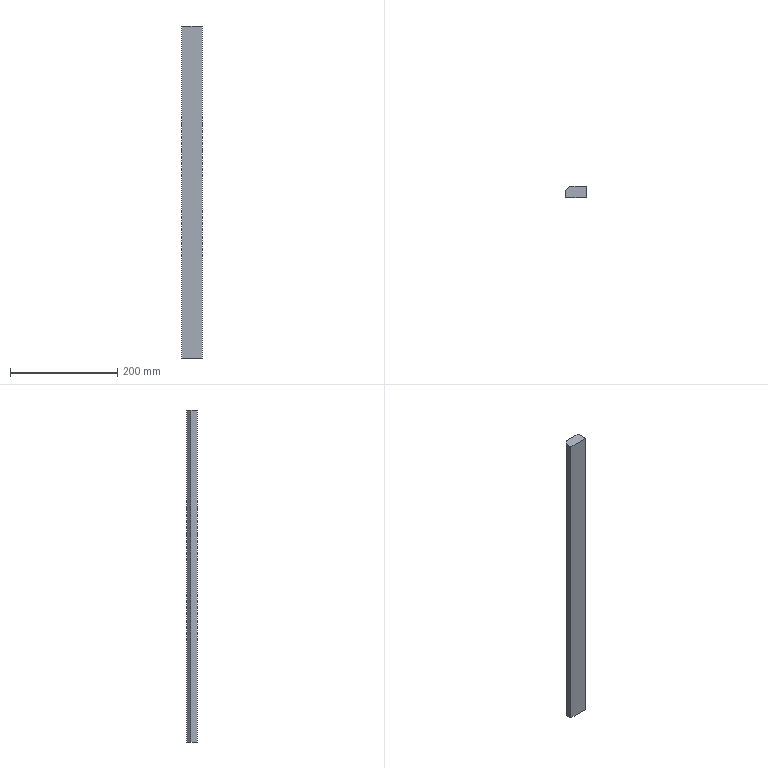Part | SolidWorks | features Chamfer 1, Extrusion 1 | 1 solid | 7 faces | box 39 x 20 x 620 mm | volume 463760 mm3 | plane 7
STEP:
#1=CARTESIAN_POINT('',(0.,12.,620.));
#2=VERTEX_POINT('',#1);
#3=CARTESIAN_POINT('',(0.,0.,620.));
#4=VERTEX_POINT('',#3);
#5=CARTESIAN_POINT('',(0.,0.,620.));
#6=DIRECTION('',(0.,-1.,0.));
#7=VECTOR('',#6,1000.);
#8=LINE('',#5,#7);
#9=EDGE_CURVE('',#2,#4,#8,.T.);
#10=ORIENTED_EDGE('',*,*,#9,.F.);
#11=CARTESIAN_POINT('',(0.,12.,0.));
#12=VERTEX_POINT('',#11);
#13=CARTESIAN_POINT('',(0.,12.,620.));
#14=DIRECTION('',(0.,0.,-1.));
#15=VECTOR('',#14,1000.);
#16=LINE('',#13,#15);
#17=EDGE_CURVE('',#2,#12,#16,.T.);
#18=ORIENTED_EDGE('',*,*,#17,.T.);
#19=CARTESIAN_POINT('',(0.,0.,0.));
#20=VERTEX_POINT('',#19);
#21=CARTESIAN_POINT('',(0.,0.,0.));
#22=DIRECTION('',(0.,-1.,0.));
#23=VECTOR('',#22,1000.);
#24=LINE('',#21,#23);
#25=EDGE_CURVE('',#12,#20,#24,.T.);
#26=ORIENTED_EDGE('',*,*,#25,.T.);
#27=CARTESIAN_POINT('',(0.,0.,620.));
#28=DIRECTION('',(0.,0.,-1.));
#29=VECTOR('',#28,1000.);
#30=LINE('',#27,#29);
#31=EDGE_CURVE('',#4,#20,#30,.T.);
#32=ORIENTED_EDGE('',*,*,#31,.F.);
#33=EDGE_LOOP('',(#10,#18,#26,#32));
#34=FACE_OUTER_BOUND('',#33,.T.);
#35=CARTESIAN_POINT('',(0.,0.,620.));
#36=DIRECTION('',(1.,0.,0.));
#37=DIRECTION('',(0.,0.,-1.));
#38=AXIS2_PLACEMENT_3D('',#35,#36,#37);
#39=PLANE('',#38);
#40=ADVANCED_FACE('',(#34),#39,.F.);
#41=CARTESIAN_POINT('',(39.,0.,0.));
#42=VERTEX_POINT('',#41);
#43=CARTESIAN_POINT('',(0.,0.,0.));
#44=DIRECTION('',(1.,0.,0.));
#45=VECTOR('',#44,1000.);
#46=LINE('',#43,#45);
#47=EDGE_CURVE('',#20,#42,#46,.T.);
#48=ORIENTED_EDGE('',*,*,#47,.T.);
#49=CARTESIAN_POINT('',(39.,0.,620.));
#50=VERTEX_POINT('',#49);
#51=CARTESIAN_POINT('',(39.,0.,620.));
#52=DIRECTION('',(0.,0.,-1.));
#53=VECTOR('',#52,1000.);
#54=LINE('',#51,#53);
#55=EDGE_CURVE('',#50,#42,#54,.T.);
#56=ORIENTED_EDGE('',*,*,#55,.F.);
#57=CARTESIAN_POINT('',(0.,0.,620.));
#58=DIRECTION('',(1.,0.,0.));
#59=VECTOR('',#58,1000.);
#60=LINE('',#57,#59);
#61=EDGE_CURVE('',#4,#50,#60,.T.);
#62=ORIENTED_EDGE('',*,*,#61,.F.);
#63=ORIENTED_EDGE('',*,*,#31,.T.);
#64=EDGE_LOOP('',(#48,#56,#62,#63));
#65=FACE_OUTER_BOUND('',#64,.T.);
#66=CARTESIAN_POINT('',(0.,0.,620.));
#67=DIRECTION('',(0.,1.,0.));
#68=DIRECTION('',(0.,0.,1.));
#69=AXIS2_PLACEMENT_3D('',#66,#67,#68);
#70=PLANE('',#69);
#71=ADVANCED_FACE('',(#65),#70,.F.);
#72=CARTESIAN_POINT('',(39.,20.,0.));
#73=VERTEX_POINT('',#72);
#74=CARTESIAN_POINT('',(39.,0.,0.));
#75=DIRECTION('',(0.,1.,0.));
#76=VECTOR('',#75,1000.);
#77=LINE('',#74,#76);
#78=EDGE_CURVE('',#42,#73,#77,.T.);
#79=ORIENTED_EDGE('',*,*,#78,.T.);
#80=CARTESIAN_POINT('',(39.,20.,620.));
#81=VERTEX_POINT('',#80);
#82=CARTESIAN_POINT('',(39.,20.,620.));
#83=DIRECTION('',(0.,0.,-1.));
#84=VECTOR('',#83,1000.);
#85=LINE('',#82,#84);
#86=EDGE_CURVE('',#81,#73,#85,.T.);
#87=ORIENTED_EDGE('',*,*,#86,.F.);
#88=CARTESIAN_POINT('',(39.,0.,620.));
#89=DIRECTION('',(0.,1.,0.));
#90=VECTOR('',#89,1000.);
#91=LINE('',#88,#90);
#92=EDGE_CURVE('',#50,#81,#91,.T.);
#93=ORIENTED_EDGE('',*,*,#92,.F.);
#94=ORIENTED_EDGE('',*,*,#55,.T.);
#95=EDGE_LOOP('',(#79,#87,#93,#94));
#96=FACE_OUTER_BOUND('',#95,.T.);
#97=CARTESIAN_POINT('',(39.,0.,620.));
#98=DIRECTION('',(-1.,0.,0.));
#99=DIRECTION('',(0.,0.,1.));
#100=AXIS2_PLACEMENT_3D('',#97,#98,#99);
#101=PLANE('',#100);
#102=ADVANCED_FACE('',(#96),#101,.F.);
#103=CARTESIAN_POINT('',(8.,20.,0.));
#104=VERTEX_POINT('',#103);
#105=CARTESIAN_POINT('',(0.,20.,0.));
#106=DIRECTION('',(-1.,0.,0.));
#107=VECTOR('',#106,1000.);
#108=LINE('',#105,#107);
#109=EDGE_CURVE('',#73,#104,#108,.T.);
#110=ORIENTED_EDGE('',*,*,#109,.T.);
#111=CARTESIAN_POINT('',(8.,20.,620.));
#112=VERTEX_POINT('',#111);
#113=CARTESIAN_POINT('',(8.,20.,620.));
#114=DIRECTION('',(0.,0.,1.));
#115=VECTOR('',#114,1000.);
#116=LINE('',#113,#115);
#117=EDGE_CURVE('',#104,#112,#116,.T.);
#118=ORIENTED_EDGE('',*,*,#117,.T.);
#119=CARTESIAN_POINT('',(0.,20.,620.));
#120=DIRECTION('',(-1.,0.,0.));
#121=VECTOR('',#120,1000.);
#122=LINE('',#119,#121);
#123=EDGE_CURVE('',#81,#112,#122,.T.);
#124=ORIENTED_EDGE('',*,*,#123,.F.);
#125=ORIENTED_EDGE('',*,*,#86,.T.);
#126=EDGE_LOOP('',(#110,#118,#124,#125));
#127=FACE_OUTER_BOUND('',#126,.T.);
#128=CARTESIAN_POINT('',(0.,20.,620.));
#129=DIRECTION('',(0.,-1.,0.));
#130=DIRECTION('',(0.,0.,-1.));
#131=AXIS2_PLACEMENT_3D('',#128,#129,#130);
#132=PLANE('',#131);
#133=ADVANCED_FACE('',(#127),#132,.F.);
#134=ORIENTED_EDGE('',*,*,#123,.T.);
#135=CARTESIAN_POINT('',(0.,12.,620.));
#136=DIRECTION('',(-0.7071,-0.7071,0.));
#137=VECTOR('',#136,1000.);
#138=LINE('',#135,#137);
#139=EDGE_CURVE('',#112,#2,#138,.T.);
#140=ORIENTED_EDGE('',*,*,#139,.T.);
#141=ORIENTED_EDGE('',*,*,#9,.T.);
#142=ORIENTED_EDGE('',*,*,#61,.T.);
#143=ORIENTED_EDGE('',*,*,#92,.T.);
#144=EDGE_LOOP('',(#134,#140,#141,#142,#143));
#145=FACE_OUTER_BOUND('',#144,.T.);
#146=CARTESIAN_POINT('',(0.,20.,620.));
#147=DIRECTION('',(0.,0.,-1.));
#148=DIRECTION('',(-1.,0.,0.));
#149=AXIS2_PLACEMENT_3D('',#146,#147,#148);
#150=PLANE('',#149);
#151=ADVANCED_FACE('',(#145),#150,.F.);
#152=ORIENTED_EDGE('',*,*,#25,.F.);
#153=CARTESIAN_POINT('',(4.,16.,0.));
#154=DIRECTION('',(0.7071,0.7071,0.));
#155=VECTOR('',#154,1000.);
#156=LINE('',#153,#155);
#157=EDGE_CURVE('',#12,#104,#156,.T.);
#158=ORIENTED_EDGE('',*,*,#157,.T.);
#159=ORIENTED_EDGE('',*,*,#109,.F.);
#160=ORIENTED_EDGE('',*,*,#78,.F.);
#161=ORIENTED_EDGE('',*,*,#47,.F.);
#162=EDGE_LOOP('',(#152,#158,#159,#160,#161));
#163=FACE_OUTER_BOUND('',#162,.T.);
#164=CARTESIAN_POINT('',(0.,20.,0.));
#165=DIRECTION('',(0.,0.,-1.));
#166=DIRECTION('',(-1.,0.,0.));
#167=AXIS2_PLACEMENT_3D('',#164,#165,#166);
#168=PLANE('',#167);
#169=ADVANCED_FACE('',(#163),#168,.T.);
#170=ORIENTED_EDGE('',*,*,#139,.F.);
#171=ORIENTED_EDGE('',*,*,#117,.F.);
#172=ORIENTED_EDGE('',*,*,#157,.F.);
#173=ORIENTED_EDGE('',*,*,#17,.F.);
#174=EDGE_LOOP('',(#170,#171,#172,#173));
#175=FACE_OUTER_BOUND('',#174,.T.);
#176=CARTESIAN_POINT('',(0.,12.,620.));
#177=DIRECTION('',(0.7071,-0.7071,0.));
#178=DIRECTION('',(0.7071,0.7071,0.));
#179=AXIS2_PLACEMENT_3D('',#176,#177,#178);
#180=PLANE('',#179);
#181=ADVANCED_FACE('',(#175),#180,.F.);
#182=CLOSED_SHELL('',(#40,#71,#102,#133,#151,#169,#181));
#183=MANIFOLD_SOLID_BREP('',#182);
#184=CARTESIAN_POINT('',(0.,0.,0.));
#185=DIRECTION('',(0.,0.,1.));
#186=DIRECTION('',(1.,0.,0.));
#187=AXIS2_PLACEMENT_3D('',#184,#185,#186);
#188=(LENGTH_UNIT()NAMED_UNIT(*)SI_UNIT(.MILLI.,.METRE.));
#189=UNCERTAINTY_MEASURE_WITH_UNIT(LENGTH_MEASURE(0.00001),#188,'','');
#190=(NAMED_UNIT(*)PLANE_ANGLE_UNIT()SI_UNIT($,.RADIAN.));
#191=(NAMED_UNIT(*)SI_UNIT($,.STERADIAN.)SOLID_ANGLE_UNIT());
#192=(GEOMETRIC_REPRESENTATION_CONTEXT(3)GLOBAL_UNCERTAINTY_ASSIGNED_CONTEXT((#189))GLOBAL_UNIT_ASSIGNED_CONTEXT((#188,#190,#191))REPRESENTATION_CONTEXT('',''));
#193=ADVANCED_BREP_SHAPE_REPRESENTATION('',(#183,#187),#192);